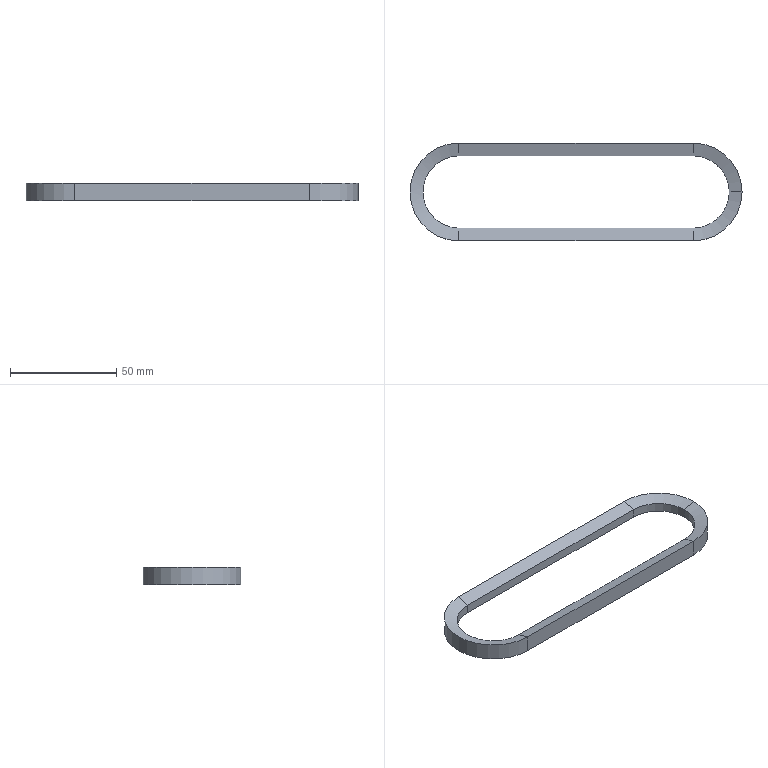Part | STEP file | Flat belt | 1 solid | 20 faces | box 156 x 46 x 8 mm | volume 12857 mm3 | plane 8 | cylinder 6 | cone 6 | commonest cylinder face diameters 34 x3 46 x3
STEP:
#1=CARTESIAN_POINT('',(127.,0.,-2.166));
#2=VERTEX_POINT('',#1);
#3=CARTESIAN_POINT('',(110.,17.,-2.166));
#4=VERTEX_POINT('',#3);
#5=CARTESIAN_POINT('',(110.,0.,-2.166));
#6=DIRECTION('',(0.,0.,1.));
#7=DIRECTION('',(0.,-1.,0.));
#8=AXIS2_PLACEMENT_3D('',#5,#6,#7);
#9=CIRCLE('',#8,17.);
#10=EDGE_CURVE('',#2,#4,#9,.T.);
#11=ORIENTED_EDGE('',*,*,#10,.F.);
#12=CARTESIAN_POINT('',(127.,0.,2.166));
#13=VERTEX_POINT('',#12);
#14=CARTESIAN_POINT('',(127.,0.,0.));
#15=DIRECTION('',(0.,0.,1.));
#16=VECTOR('',#15,1000.);
#17=LINE('',#14,#16);
#18=EDGE_CURVE('',#2,#13,#17,.T.);
#19=ORIENTED_EDGE('',*,*,#18,.T.);
#20=CARTESIAN_POINT('',(110.,17.,2.166));
#21=VERTEX_POINT('',#20);
#22=CARTESIAN_POINT('',(110.,0.,2.166));
#23=DIRECTION('',(0.,0.,1.));
#24=DIRECTION('',(0.,-1.,0.));
#25=AXIS2_PLACEMENT_3D('',#22,#23,#24);
#26=CIRCLE('',#25,17.);
#27=EDGE_CURVE('',#13,#21,#26,.T.);
#28=ORIENTED_EDGE('',*,*,#27,.T.);
#29=CARTESIAN_POINT('',(110.,17.,2.166));
#30=DIRECTION('',(0.,0.,-1.));
#31=VECTOR('',#30,1000.);
#32=LINE('',#29,#31);
#33=EDGE_CURVE('',#21,#4,#32,.T.);
#34=ORIENTED_EDGE('',*,*,#33,.T.);
#35=EDGE_LOOP('',(#11,#19,#28,#34));
#36=FACE_OUTER_BOUND('',#35,.T.);
#37=CARTESIAN_POINT('',(110.,0.,0.));
#38=DIRECTION('',(0.,0.,1.));
#39=DIRECTION('',(1.,0.,0.));
#40=AXIS2_PLACEMENT_3D('',#37,#38,#39);
#41=CYLINDRICAL_SURFACE('',#40,17.);
#42=ADVANCED_FACE('',(#36),#41,.F.);
#43=ORIENTED_EDGE('',*,*,#27,.F.);
#44=CARTESIAN_POINT('',(133.,0.,4.));
#45=VERTEX_POINT('',#44);
#46=CARTESIAN_POINT('',(133.,0.,4.));
#47=DIRECTION('',(0.9563,0.,0.2924));
#48=VECTOR('',#47,1000.);
#49=LINE('',#46,#48);
#50=EDGE_CURVE('',#13,#45,#49,.T.);
#51=ORIENTED_EDGE('',*,*,#50,.T.);
#52=CARTESIAN_POINT('',(110.,23.,4.));
#53=VERTEX_POINT('',#52);
#54=CARTESIAN_POINT('',(110.,0.,4.));
#55=DIRECTION('',(0.,0.,1.));
#56=DIRECTION('',(0.,-1.,0.));
#57=AXIS2_PLACEMENT_3D('',#54,#55,#56);
#58=CIRCLE('',#57,23.);
#59=EDGE_CURVE('',#45,#53,#58,.T.);
#60=ORIENTED_EDGE('',*,*,#59,.T.);
#61=CARTESIAN_POINT('',(110.,17.,2.166));
#62=DIRECTION('',(0.,-0.9563,-0.2924));
#63=VECTOR('',#62,1000.);
#64=LINE('',#61,#63);
#65=EDGE_CURVE('',#53,#21,#64,.T.);
#66=ORIENTED_EDGE('',*,*,#65,.T.);
#67=EDGE_LOOP('',(#43,#51,#60,#66));
#68=FACE_OUTER_BOUND('',#67,.T.);
#69=CARTESIAN_POINT('',(110.,0.,4.));
#70=DIRECTION('',(0.,0.,1.));
#71=DIRECTION('',(1.,0.,0.));
#72=AXIS2_PLACEMENT_3D('',#69,#70,#71);
#73=CONICAL_SURFACE('',#72,23.,1.274);
#74=ADVANCED_FACE('',(#68),#73,.F.);
#75=CARTESIAN_POINT('',(110.,-23.,-4.));
#76=VERTEX_POINT('',#75);
#77=CARTESIAN_POINT('',(133.,0.,-4.));
#78=VERTEX_POINT('',#77);
#79=CARTESIAN_POINT('',(110.,0.,-4.));
#80=DIRECTION('',(0.,0.,1.));
#81=DIRECTION('',(0.,-1.,0.));
#82=AXIS2_PLACEMENT_3D('',#79,#80,#81);
#83=CIRCLE('',#82,23.);
#84=EDGE_CURVE('',#76,#78,#83,.T.);
#85=ORIENTED_EDGE('',*,*,#84,.T.);
#86=CARTESIAN_POINT('',(133.,0.,0.));
#87=DIRECTION('',(0.,0.,1.));
#88=VECTOR('',#87,1000.);
#89=LINE('',#86,#88);
#90=EDGE_CURVE('',#78,#45,#89,.T.);
#91=ORIENTED_EDGE('',*,*,#90,.T.);
#92=CARTESIAN_POINT('',(110.,-23.,4.));
#93=VERTEX_POINT('',#92);
#94=CARTESIAN_POINT('',(110.,0.,4.));
#95=DIRECTION('',(0.,0.,1.));
#96=DIRECTION('',(0.,-1.,0.));
#97=AXIS2_PLACEMENT_3D('',#94,#95,#96);
#98=CIRCLE('',#97,23.);
#99=EDGE_CURVE('',#93,#45,#98,.T.);
#100=ORIENTED_EDGE('',*,*,#99,.F.);
#101=CARTESIAN_POINT('',(110.,-23.,-4.));
#102=DIRECTION('',(0.,0.,1.));
#103=VECTOR('',#102,1000.);
#104=LINE('',#101,#103);
#105=EDGE_CURVE('',#76,#93,#104,.T.);
#106=ORIENTED_EDGE('',*,*,#105,.F.);
#107=EDGE_LOOP('',(#85,#91,#100,#106));
#108=FACE_OUTER_BOUND('',#107,.T.);
#109=CARTESIAN_POINT('',(110.,0.,0.));
#110=DIRECTION('',(0.,0.,1.));
#111=DIRECTION('',(1.,0.,0.));
#112=AXIS2_PLACEMENT_3D('',#109,#110,#111);
#113=CYLINDRICAL_SURFACE('',#112,23.);
#114=ADVANCED_FACE('',(#108),#113,.T.);
#115=CARTESIAN_POINT('',(0.,17.,-2.166));
#116=VERTEX_POINT('',#115);
#117=CARTESIAN_POINT('',(-17.,0.,-2.166));
#118=VERTEX_POINT('',#117);
#119=CARTESIAN_POINT('',(0.,0.,-2.166));
#120=DIRECTION('',(0.,0.,1.));
#121=DIRECTION('',(0.,1.,0.));
#122=AXIS2_PLACEMENT_3D('',#119,#120,#121);
#123=CIRCLE('',#122,17.);
#124=EDGE_CURVE('',#116,#118,#123,.T.);
#125=ORIENTED_EDGE('',*,*,#124,.T.);
#126=CARTESIAN_POINT('',(-23.,0.,-4.));
#127=VERTEX_POINT('',#126);
#128=CARTESIAN_POINT('',(-17.,0.,-2.166));
#129=DIRECTION('',(-0.9563,0.,-0.2924));
#130=VECTOR('',#129,1000.);
#131=LINE('',#128,#130);
#132=EDGE_CURVE('',#118,#127,#131,.T.);
#133=ORIENTED_EDGE('',*,*,#132,.T.);
#134=CARTESIAN_POINT('',(0.,23.,-4.));
#135=VERTEX_POINT('',#134);
#136=CARTESIAN_POINT('',(0.,0.,-4.));
#137=DIRECTION('',(0.,0.,1.));
#138=DIRECTION('',(0.,1.,0.));
#139=AXIS2_PLACEMENT_3D('',#136,#137,#138);
#140=CIRCLE('',#139,23.);
#141=EDGE_CURVE('',#135,#127,#140,.T.);
#142=ORIENTED_EDGE('',*,*,#141,.F.);
#143=CARTESIAN_POINT('',(0.,17.,-2.166));
#144=DIRECTION('',(0.,0.9563,-0.2924));
#145=VECTOR('',#144,1000.);
#146=LINE('',#143,#145);
#147=EDGE_CURVE('',#116,#135,#146,.T.);
#148=ORIENTED_EDGE('',*,*,#147,.F.);
#149=EDGE_LOOP('',(#125,#133,#142,#148));
#150=FACE_OUTER_BOUND('',#149,.T.);
#151=CARTESIAN_POINT('',(0.,0.,-2.166));
#152=DIRECTION('',(0.,0.,-1.));
#153=DIRECTION('',(-1.,0.,0.));
#154=AXIS2_PLACEMENT_3D('',#151,#152,#153);
#155=CONICAL_SURFACE('',#154,17.,1.274);
#156=ADVANCED_FACE('',(#150),#155,.F.);
#157=CARTESIAN_POINT('',(110.,23.,-4.));
#158=VERTEX_POINT('',#157);
#159=CARTESIAN_POINT('',(110.,17.,-2.166));
#160=DIRECTION('',(0.,0.9563,-0.2924));
#161=VECTOR('',#160,1000.);
#162=LINE('',#159,#161);
#163=EDGE_CURVE('',#4,#158,#162,.T.);
#164=ORIENTED_EDGE('',*,*,#163,.F.);
#165=CARTESIAN_POINT('',(110.,17.,-2.166));
#166=DIRECTION('',(-1.,0.,0.));
#167=VECTOR('',#166,1000.);
#168=LINE('',#165,#167);
#169=EDGE_CURVE('',#4,#116,#168,.T.);
#170=ORIENTED_EDGE('',*,*,#169,.T.);
#171=ORIENTED_EDGE('',*,*,#147,.T.);
#172=CARTESIAN_POINT('',(110.,23.,-4.));
#173=DIRECTION('',(-1.,0.,0.));
#174=VECTOR('',#173,1000.);
#175=LINE('',#172,#174);
#176=EDGE_CURVE('',#158,#135,#175,.T.);
#177=ORIENTED_EDGE('',*,*,#176,.F.);
#178=EDGE_LOOP('',(#164,#170,#171,#177));
#179=FACE_OUTER_BOUND('',#178,.T.);
#180=CARTESIAN_POINT('',(110.,17.,-2.166));
#181=DIRECTION('',(0.,0.2924,0.9563));
#182=DIRECTION('',(0.,-0.9563,0.2924));
#183=AXIS2_PLACEMENT_3D('',#180,#181,#182);
#184=PLANE('',#183);
#185=ADVANCED_FACE('',(#179),#184,.F.);
#186=ORIENTED_EDGE('',*,*,#132,.F.);
#187=CARTESIAN_POINT('',(0.,-17.,-2.166));
#188=VERTEX_POINT('',#187);
#189=CARTESIAN_POINT('',(0.,0.,-2.166));
#190=DIRECTION('',(0.,0.,1.));
#191=DIRECTION('',(0.,1.,0.));
#192=AXIS2_PLACEMENT_3D('',#189,#190,#191);
#193=CIRCLE('',#192,17.);
#194=EDGE_CURVE('',#118,#188,#193,.T.);
#195=ORIENTED_EDGE('',*,*,#194,.T.);
#196=CARTESIAN_POINT('',(0.,-23.,-4.));
#197=VERTEX_POINT('',#196);
#198=CARTESIAN_POINT('',(0.,-17.,-2.166));
#199=DIRECTION('',(0.,-0.9563,-0.2924));
#200=VECTOR('',#199,1000.);
#201=LINE('',#198,#200);
#202=EDGE_CURVE('',#188,#197,#201,.T.);
#203=ORIENTED_EDGE('',*,*,#202,.T.);
#204=CARTESIAN_POINT('',(0.,0.,-4.));
#205=DIRECTION('',(0.,0.,1.));
#206=DIRECTION('',(0.,1.,0.));
#207=AXIS2_PLACEMENT_3D('',#204,#205,#206);
#208=CIRCLE('',#207,23.);
#209=EDGE_CURVE('',#127,#197,#208,.T.);
#210=ORIENTED_EDGE('',*,*,#209,.F.);
#211=EDGE_LOOP('',(#186,#195,#203,#210));
#212=FACE_OUTER_BOUND('',#211,.T.);
#213=CARTESIAN_POINT('',(0.,0.,-2.166));
#214=DIRECTION('',(0.,0.,-1.));
#215=DIRECTION('',(-1.,0.,0.));
#216=AXIS2_PLACEMENT_3D('',#213,#214,#215);
#217=CONICAL_SURFACE('',#216,17.,1.274);
#218=ADVANCED_FACE('',(#212),#217,.F.);
#219=CARTESIAN_POINT('',(0.,23.,4.));
#220=VERTEX_POINT('',#219);
#221=CARTESIAN_POINT('',(0.,-23.,4.));
#222=VERTEX_POINT('',#221);
#223=CARTESIAN_POINT('',(0.,0.,4.));
#224=DIRECTION('',(0.,0.,1.));
#225=DIRECTION('',(0.,1.,0.));
#226=AXIS2_PLACEMENT_3D('',#223,#224,#225);
#227=CIRCLE('',#226,23.);
#228=EDGE_CURVE('',#220,#222,#227,.T.);
#229=ORIENTED_EDGE('',*,*,#228,.F.);
#230=CARTESIAN_POINT('',(0.,23.,-4.));
#231=DIRECTION('',(0.,0.,1.));
#232=VECTOR('',#231,1000.);
#233=LINE('',#230,#232);
#234=EDGE_CURVE('',#135,#220,#233,.T.);
#235=ORIENTED_EDGE('',*,*,#234,.F.);
#236=ORIENTED_EDGE('',*,*,#141,.T.);
#237=ORIENTED_EDGE('',*,*,#209,.T.);
#238=CARTESIAN_POINT('',(0.,-23.,-4.));
#239=DIRECTION('',(0.,0.,1.));
#240=VECTOR('',#239,1000.);
#241=LINE('',#238,#240);
#242=EDGE_CURVE('',#197,#222,#241,.T.);
#243=ORIENTED_EDGE('',*,*,#242,.T.);
#244=EDGE_LOOP('',(#229,#235,#236,#237,#243));
#245=FACE_OUTER_BOUND('',#244,.T.);
#246=CARTESIAN_POINT('',(0.,0.,0.));
#247=DIRECTION('',(0.,0.,1.));
#248=DIRECTION('',(1.,0.,0.));
#249=AXIS2_PLACEMENT_3D('',#246,#247,#248);
#250=CYLINDRICAL_SURFACE('',#249,23.);
#251=ADVANCED_FACE('',(#245),#250,.T.);
#252=CARTESIAN_POINT('',(0.,17.,2.166));
#253=VERTEX_POINT('',#252);
#254=CARTESIAN_POINT('',(0.,-17.,2.166));
#255=VERTEX_POINT('',#254);
#256=CARTESIAN_POINT('',(0.,0.,2.166));
#257=DIRECTION('',(0.,0.,1.));
#258=DIRECTION('',(0.,1.,0.));
#259=AXIS2_PLACEMENT_3D('',#256,#257,#258);
#260=CIRCLE('',#259,17.);
#261=EDGE_CURVE('',#253,#255,#260,.T.);
#262=ORIENTED_EDGE('',*,*,#261,.F.);
#263=CARTESIAN_POINT('',(0.,17.,2.166));
#264=DIRECTION('',(0.,-0.9563,-0.2924));
#265=VECTOR('',#264,1000.);
#266=LINE('',#263,#265);
#267=EDGE_CURVE('',#220,#253,#266,.T.);
#268=ORIENTED_EDGE('',*,*,#267,.F.);
#269=ORIENTED_EDGE('',*,*,#228,.T.);
#270=CARTESIAN_POINT('',(0.,-17.,2.166));
#271=DIRECTION('',(0.,0.9563,-0.2924));
#272=VECTOR('',#271,1000.);
#273=LINE('',#270,#272);
#274=EDGE_CURVE('',#222,#255,#273,.T.);
#275=ORIENTED_EDGE('',*,*,#274,.T.);
#276=EDGE_LOOP('',(#262,#268,#269,#275));
#277=FACE_OUTER_BOUND('',#276,.T.);
#278=CARTESIAN_POINT('',(0.,0.,4.));
#279=DIRECTION('',(0.,0.,1.));
#280=DIRECTION('',(1.,0.,0.));
#281=AXIS2_PLACEMENT_3D('',#278,#279,#280);
#282=CONICAL_SURFACE('',#281,23.,1.274);
#283=ADVANCED_FACE('',(#277),#282,.F.);
#284=CARTESIAN_POINT('',(0.,-17.,2.166));
#285=DIRECTION('',(0.,0.,-1.));
#286=VECTOR('',#285,1000.);
#287=LINE('',#284,#286);
#288=EDGE_CURVE('',#255,#188,#287,.T.);
#289=ORIENTED_EDGE('',*,*,#288,.T.);
#290=ORIENTED_EDGE('',*,*,#194,.F.);
#291=ORIENTED_EDGE('',*,*,#124,.F.);
#292=CARTESIAN_POINT('',(0.,17.,2.166));
#293=DIRECTION('',(0.,0.,-1.));
#294=VECTOR('',#293,1000.);
#295=LINE('',#292,#294);
#296=EDGE_CURVE('',#253,#116,#295,.T.);
#297=ORIENTED_EDGE('',*,*,#296,.F.);
#298=ORIENTED_EDGE('',*,*,#261,.T.);
#299=EDGE_LOOP('',(#289,#290,#291,#297,#298));
#300=FACE_OUTER_BOUND('',#299,.T.);
#301=CARTESIAN_POINT('',(0.,0.,0.));
#302=DIRECTION('',(0.,0.,1.));
#303=DIRECTION('',(1.,0.,0.));
#304=AXIS2_PLACEMENT_3D('',#301,#302,#303);
#305=CYLINDRICAL_SURFACE('',#304,17.);
#306=ADVANCED_FACE('',(#300),#305,.F.);
#307=CARTESIAN_POINT('',(0.,-23.,-4.));
#308=DIRECTION('',(1.,0.,0.));
#309=VECTOR('',#308,1000.);
#310=LINE('',#307,#309);
#311=EDGE_CURVE('',#197,#76,#310,.T.);
#312=ORIENTED_EDGE('',*,*,#311,.F.);
#313=ORIENTED_EDGE('',*,*,#202,.F.);
#314=CARTESIAN_POINT('',(110.,-17.,-2.166));
#315=VERTEX_POINT('',#314);
#316=CARTESIAN_POINT('',(0.,-17.,-2.166));
#317=DIRECTION('',(1.,0.,0.));
#318=VECTOR('',#317,1000.);
#319=LINE('',#316,#318);
#320=EDGE_CURVE('',#188,#315,#319,.T.);
#321=ORIENTED_EDGE('',*,*,#320,.T.);
#322=CARTESIAN_POINT('',(110.,-17.,-2.166));
#323=DIRECTION('',(0.,-0.9563,-0.2924));
#324=VECTOR('',#323,1000.);
#325=LINE('',#322,#324);
#326=EDGE_CURVE('',#315,#76,#325,.T.);
#327=ORIENTED_EDGE('',*,*,#326,.T.);
#328=EDGE_LOOP('',(#312,#313,#321,#327));
#329=FACE_OUTER_BOUND('',#328,.T.);
#330=CARTESIAN_POINT('',(0.,-17.,-2.166));
#331=DIRECTION('',(0.,-0.2924,0.9563));
#332=DIRECTION('',(0.,-0.9563,-0.2924));
#333=AXIS2_PLACEMENT_3D('',#330,#331,#332);
#334=PLANE('',#333);
#335=ADVANCED_FACE('',(#329),#334,.F.);
#336=CARTESIAN_POINT('',(0.,-23.,4.));
#337=DIRECTION('',(1.,0.,0.));
#338=VECTOR('',#337,1000.);
#339=LINE('',#336,#338);
#340=EDGE_CURVE('',#222,#93,#339,.T.);
#341=ORIENTED_EDGE('',*,*,#340,.F.);
#342=ORIENTED_EDGE('',*,*,#242,.F.);
#343=ORIENTED_EDGE('',*,*,#311,.T.);
#344=ORIENTED_EDGE('',*,*,#105,.T.);
#345=EDGE_LOOP('',(#341,#342,#343,#344));
#346=FACE_OUTER_BOUND('',#345,.T.);
#347=CARTESIAN_POINT('',(0.,-23.,-4.));
#348=DIRECTION('',(0.,1.,0.));
#349=DIRECTION('',(-1.,0.,0.));
#350=AXIS2_PLACEMENT_3D('',#347,#348,#349);
#351=PLANE('',#350);
#352=ADVANCED_FACE('',(#346),#351,.F.);
#353=CARTESIAN_POINT('',(110.,-17.,2.166));
#354=VERTEX_POINT('',#353);
#355=CARTESIAN_POINT('',(0.,-17.,2.166));
#356=DIRECTION('',(1.,0.,0.));
#357=VECTOR('',#356,1000.);
#358=LINE('',#355,#357);
#359=EDGE_CURVE('',#255,#354,#358,.T.);
#360=ORIENTED_EDGE('',*,*,#359,.F.);
#361=ORIENTED_EDGE('',*,*,#274,.F.);
#362=ORIENTED_EDGE('',*,*,#340,.T.);
#363=CARTESIAN_POINT('',(110.,-17.,2.166));
#364=DIRECTION('',(0.,0.9563,-0.2924));
#365=VECTOR('',#364,1000.);
#366=LINE('',#363,#365);
#367=EDGE_CURVE('',#93,#354,#366,.T.);
#368=ORIENTED_EDGE('',*,*,#367,.T.);
#369=EDGE_LOOP('',(#360,#361,#362,#368));
#370=FACE_OUTER_BOUND('',#369,.T.);
#371=CARTESIAN_POINT('',(0.,-17.,2.166));
#372=DIRECTION('',(0.,-0.2924,-0.9563));
#373=DIRECTION('',(0.,0.9563,-0.2924));
#374=AXIS2_PLACEMENT_3D('',#371,#372,#373);
#375=PLANE('',#374);
#376=ADVANCED_FACE('',(#370),#375,.F.);
#377=CARTESIAN_POINT('',(110.,-17.,2.166));
#378=DIRECTION('',(0.,0.,-1.));
#379=VECTOR('',#378,1000.);
#380=LINE('',#377,#379);
#381=EDGE_CURVE('',#354,#315,#380,.T.);
#382=ORIENTED_EDGE('',*,*,#381,.T.);
#383=ORIENTED_EDGE('',*,*,#320,.F.);
#384=ORIENTED_EDGE('',*,*,#288,.F.);
#385=ORIENTED_EDGE('',*,*,#359,.T.);
#386=EDGE_LOOP('',(#382,#383,#384,#385));
#387=FACE_OUTER_BOUND('',#386,.T.);
#388=CARTESIAN_POINT('',(0.,-17.,2.166));
#389=DIRECTION('',(0.,-1.,0.));
#390=DIRECTION('',(1.,0.,0.));
#391=AXIS2_PLACEMENT_3D('',#388,#389,#390);
#392=PLANE('',#391);
#393=ADVANCED_FACE('',(#387),#392,.F.);
#394=ORIENTED_EDGE('',*,*,#84,.F.);
#395=ORIENTED_EDGE('',*,*,#326,.F.);
#396=CARTESIAN_POINT('',(110.,0.,-2.166));
#397=DIRECTION('',(0.,0.,1.));
#398=DIRECTION('',(0.,-1.,0.));
#399=AXIS2_PLACEMENT_3D('',#396,#397,#398);
#400=CIRCLE('',#399,17.);
#401=EDGE_CURVE('',#315,#2,#400,.T.);
#402=ORIENTED_EDGE('',*,*,#401,.T.);
#403=ORIENTED_EDGE('',*,*,#10,.T.);
#404=ORIENTED_EDGE('',*,*,#163,.T.);
#405=CARTESIAN_POINT('',(110.,0.,-4.));
#406=DIRECTION('',(0.,0.,1.));
#407=DIRECTION('',(0.,-1.,0.));
#408=AXIS2_PLACEMENT_3D('',#405,#406,#407);
#409=CIRCLE('',#408,23.);
#410=EDGE_CURVE('',#78,#158,#409,.T.);
#411=ORIENTED_EDGE('',*,*,#410,.F.);
#412=EDGE_LOOP('',(#394,#395,#402,#403,#404,#411));
#413=FACE_OUTER_BOUND('',#412,.T.);
#414=CARTESIAN_POINT('',(110.,0.,-2.166));
#415=DIRECTION('',(0.,0.,-1.));
#416=DIRECTION('',(-1.,0.,0.));
#417=AXIS2_PLACEMENT_3D('',#414,#415,#416);
#418=CONICAL_SURFACE('',#417,17.,1.274);
#419=ADVANCED_FACE('',(#413),#418,.F.);
#420=ORIENTED_EDGE('',*,*,#90,.F.);
#421=ORIENTED_EDGE('',*,*,#410,.T.);
#422=CARTESIAN_POINT('',(110.,23.,-4.));
#423=DIRECTION('',(0.,0.,1.));
#424=VECTOR('',#423,1000.);
#425=LINE('',#422,#424);
#426=EDGE_CURVE('',#158,#53,#425,.T.);
#427=ORIENTED_EDGE('',*,*,#426,.T.);
#428=ORIENTED_EDGE('',*,*,#59,.F.);
#429=EDGE_LOOP('',(#420,#421,#427,#428));
#430=FACE_OUTER_BOUND('',#429,.T.);
#431=CARTESIAN_POINT('',(110.,0.,0.));
#432=DIRECTION('',(0.,0.,1.));
#433=DIRECTION('',(1.,0.,0.));
#434=AXIS2_PLACEMENT_3D('',#431,#432,#433);
#435=CYLINDRICAL_SURFACE('',#434,23.);
#436=ADVANCED_FACE('',(#430),#435,.T.);
#437=ORIENTED_EDGE('',*,*,#50,.F.);
#438=CARTESIAN_POINT('',(110.,0.,2.166));
#439=DIRECTION('',(0.,0.,1.));
#440=DIRECTION('',(0.,-1.,0.));
#441=AXIS2_PLACEMENT_3D('',#438,#439,#440);
#442=CIRCLE('',#441,17.);
#443=EDGE_CURVE('',#354,#13,#442,.T.);
#444=ORIENTED_EDGE('',*,*,#443,.F.);
#445=ORIENTED_EDGE('',*,*,#367,.F.);
#446=ORIENTED_EDGE('',*,*,#99,.T.);
#447=EDGE_LOOP('',(#437,#444,#445,#446));
#448=FACE_OUTER_BOUND('',#447,.T.);
#449=CARTESIAN_POINT('',(110.,0.,4.));
#450=DIRECTION('',(0.,0.,1.));
#451=DIRECTION('',(1.,0.,0.));
#452=AXIS2_PLACEMENT_3D('',#449,#450,#451);
#453=CONICAL_SURFACE('',#452,23.,1.274);
#454=ADVANCED_FACE('',(#448),#453,.F.);
#455=ORIENTED_EDGE('',*,*,#18,.F.);
#456=ORIENTED_EDGE('',*,*,#401,.F.);
#457=ORIENTED_EDGE('',*,*,#381,.F.);
#458=ORIENTED_EDGE('',*,*,#443,.T.);
#459=EDGE_LOOP('',(#455,#456,#457,#458));
#460=FACE_OUTER_BOUND('',#459,.T.);
#461=CARTESIAN_POINT('',(110.,0.,0.));
#462=DIRECTION('',(0.,0.,1.));
#463=DIRECTION('',(1.,0.,0.));
#464=AXIS2_PLACEMENT_3D('',#461,#462,#463);
#465=CYLINDRICAL_SURFACE('',#464,17.);
#466=ADVANCED_FACE('',(#460),#465,.F.);
#467=ORIENTED_EDGE('',*,*,#176,.T.);
#468=ORIENTED_EDGE('',*,*,#234,.T.);
#469=CARTESIAN_POINT('',(110.,23.,4.));
#470=DIRECTION('',(-1.,0.,0.));
#471=VECTOR('',#470,1000.);
#472=LINE('',#469,#471);
#473=EDGE_CURVE('',#53,#220,#472,.T.);
#474=ORIENTED_EDGE('',*,*,#473,.F.);
#475=ORIENTED_EDGE('',*,*,#426,.F.);
#476=EDGE_LOOP('',(#467,#468,#474,#475));
#477=FACE_OUTER_BOUND('',#476,.T.);
#478=CARTESIAN_POINT('',(110.,23.,-4.));
#479=DIRECTION('',(0.,-1.,0.));
#480=DIRECTION('',(1.,0.,0.));
#481=AXIS2_PLACEMENT_3D('',#478,#479,#480);
#482=PLANE('',#481);
#483=ADVANCED_FACE('',(#477),#482,.F.);
#484=ORIENTED_EDGE('',*,*,#473,.T.);
#485=ORIENTED_EDGE('',*,*,#267,.T.);
#486=CARTESIAN_POINT('',(110.,17.,2.166));
#487=DIRECTION('',(-1.,0.,0.));
#488=VECTOR('',#487,1000.);
#489=LINE('',#486,#488);
#490=EDGE_CURVE('',#21,#253,#489,.T.);
#491=ORIENTED_EDGE('',*,*,#490,.F.);
#492=ORIENTED_EDGE('',*,*,#65,.F.);
#493=EDGE_LOOP('',(#484,#485,#491,#492));
#494=FACE_OUTER_BOUND('',#493,.T.);
#495=CARTESIAN_POINT('',(110.,17.,2.166));
#496=DIRECTION('',(0.,0.2924,-0.9563));
#497=DIRECTION('',(0.,0.9563,0.2924));
#498=AXIS2_PLACEMENT_3D('',#495,#496,#497);
#499=PLANE('',#498);
#500=ADVANCED_FACE('',(#494),#499,.F.);
#501=ORIENTED_EDGE('',*,*,#490,.T.);
#502=ORIENTED_EDGE('',*,*,#296,.T.);
#503=ORIENTED_EDGE('',*,*,#169,.F.);
#504=ORIENTED_EDGE('',*,*,#33,.F.);
#505=EDGE_LOOP('',(#501,#502,#503,#504));
#506=FACE_OUTER_BOUND('',#505,.T.);
#507=CARTESIAN_POINT('',(110.,17.,2.166));
#508=DIRECTION('',(0.,1.,0.));
#509=DIRECTION('',(-1.,0.,0.));
#510=AXIS2_PLACEMENT_3D('',#507,#508,#509);
#511=PLANE('',#510);
#512=ADVANCED_FACE('',(#506),#511,.F.);
#513=CLOSED_SHELL('',(#42,#74,#114,#156,#185,#218,#251,#283,#306,#335,#352,#376,#393,#419,#436,#454,#466,#483,#500,#512));
#514=MANIFOLD_SOLID_BREP('',#513);
#515=CARTESIAN_POINT('',(0.,0.,0.));
#516=DIRECTION('',(0.,0.,1.));
#517=DIRECTION('',(1.,0.,0.));
#518=AXIS2_PLACEMENT_3D('',#515,#516,#517);
#519=(LENGTH_UNIT()NAMED_UNIT(*)SI_UNIT(.MILLI.,.METRE.));
#520=UNCERTAINTY_MEASURE_WITH_UNIT(LENGTH_MEASURE(0.00001),#519,'','');
#521=(NAMED_UNIT(*)PLANE_ANGLE_UNIT()SI_UNIT($,.RADIAN.));
#522=(NAMED_UNIT(*)SI_UNIT($,.STERADIAN.)SOLID_ANGLE_UNIT());
#523=(GEOMETRIC_REPRESENTATION_CONTEXT(3)GLOBAL_UNCERTAINTY_ASSIGNED_CONTEXT((#520))GLOBAL_UNIT_ASSIGNED_CONTEXT((#519,#521,#522))REPRESENTATION_CONTEXT('',''));
#524=ADVANCED_BREP_SHAPE_REPRESENTATION('',(#514,#518),#523);